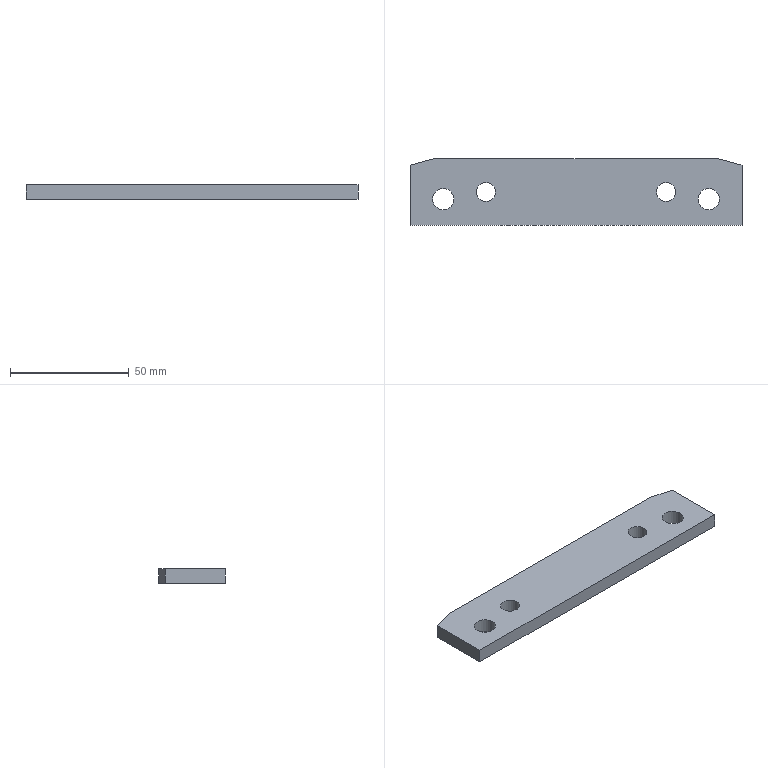Part | STEP file | gslz 2016.10.28-13_id738_x_t | 1 solid | 12 faces | box 140 x 28 x 6 mm | volume 21993 mm3 | plane 8 | cylinder 4 | commonest cylinder face diameters 8 x2 9 x2
STEP:
#1=CARTESIAN_POINT('',(0.,0.,0.));
#2=DIRECTION('',(0.,0.,1.));
#3=DIRECTION('',(1.,0.,0.));
#4=AXIS2_PLACEMENT_3D('',#1,#2,#3);
#5=CARTESIAN_POINT('',(135.484,-281.75,6.));
#6=VERTEX_POINT('',#5);
#7=CARTESIAN_POINT('',(143.484,-281.75,6.));
#8=VERTEX_POINT('',#7);
#9=CARTESIAN_POINT('',(139.484,-281.75,6.));
#10=DIRECTION('',(0.,0.,-1.));
#11=DIRECTION('',(-1.,0.,0.));
#12=AXIS2_PLACEMENT_3D('',#9,#10,#11);
#13=CIRCLE('',#12,4.);
#14=CARTESIAN_POINT('',(139.484,-281.75,-73.));
#15=DIRECTION('',(0.,0.,1.));
#16=DIRECTION('',(1.,0.,0.));
#17=AXIS2_PLACEMENT_3D('',#14,#15,#16);
#18=CYLINDRICAL_SURFACE('',#17,4.);
#19=CARTESIAN_POINT('',(3.142,79.));
#20=DIRECTION('',(-1.,0.));
#21=VECTOR('',#20,1.);
#22=LINE('',#19,#21);
#23=(GEOMETRIC_REPRESENTATION_CONTEXT(2)PARAMETRIC_REPRESENTATION_CONTEXT()REPRESENTATION_CONTEXT('',''));
#24=DEFINITIONAL_REPRESENTATION('',(#22),#23);
#25=PCURVE('',#18,#24);
#26=CARTESIAN_POINT('',(142.484,-265.25,6.));
#27=DIRECTION('',(0.,0.,-1.));
#28=DIRECTION('',(-1.,0.,0.));
#29=AXIS2_PLACEMENT_3D('',#26,#27,#28);
#30=PLANE('',#29);
#31=CARTESIAN_POINT('',(3.,-16.5));
#32=DIRECTION('',(1.,0.));
#33=AXIS2_PLACEMENT_2D('',#31,#32);
#34=CIRCLE('',#33,4.);
#35=(GEOMETRIC_REPRESENTATION_CONTEXT(2)PARAMETRIC_REPRESENTATION_CONTEXT()REPRESENTATION_CONTEXT('',''));
#36=DEFINITIONAL_REPRESENTATION('',(#34),#35);
#37=PCURVE('',#30,#36);
#38=SURFACE_CURVE('',#13,(#25,#37),.PCURVE_S1.);
#39=EDGE_CURVE('',#6,#8,#38,.T.);
#40=ORIENTED_EDGE('',*,*,#39,.T.);
#41=CARTESIAN_POINT('',(143.484,-281.75,0.));
#42=VERTEX_POINT('',#41);
#43=CARTESIAN_POINT('',(143.484,-281.75,0.));
#44=CARTESIAN_POINT('',(143.484,-281.75,6.));
#45=B_SPLINE_CURVE_WITH_KNOTS('',1,(#43,#44),.UNSPECIFIED.,.F.,.F.,(2,2),(73.,79.),.PIECEWISE_BEZIER_KNOTS.);
#46=CARTESIAN_POINT('',(0.,0.));
#47=DIRECTION('',(0.,1.));
#48=VECTOR('',#47,1.);
#49=LINE('',#46,#48);
#50=(GEOMETRIC_REPRESENTATION_CONTEXT(2)PARAMETRIC_REPRESENTATION_CONTEXT()REPRESENTATION_CONTEXT('',''));
#51=DEFINITIONAL_REPRESENTATION('',(#49),#50);
#52=PCURVE('',#18,#51);
#53=CARTESIAN_POINT('',(6.283,0.));
#54=DIRECTION('',(0.,1.));
#55=VECTOR('',#54,1.);
#56=LINE('',#53,#55);
#57=(GEOMETRIC_REPRESENTATION_CONTEXT(2)PARAMETRIC_REPRESENTATION_CONTEXT()REPRESENTATION_CONTEXT('',''));
#58=DEFINITIONAL_REPRESENTATION('',(#56),#57);
#59=PCURVE('',#18,#58);
#60=SEAM_CURVE('',#45,(#52,#59),.PCURVE_S1.);
#61=EDGE_CURVE('',#42,#8,#60,.T.);
#62=ORIENTED_EDGE('',*,*,#61,.F.);
#63=CARTESIAN_POINT('',(139.484,-281.75,0.));
#64=DIRECTION('',(0.,0.,1.));
#65=DIRECTION('',(1.,0.,0.));
#66=AXIS2_PLACEMENT_3D('',#63,#64,#65);
#67=CIRCLE('',#66,4.);
#68=CARTESIAN_POINT('',(0.,73.));
#69=DIRECTION('',(1.,0.));
#70=VECTOR('',#69,1.);
#71=LINE('',#68,#70);
#72=(GEOMETRIC_REPRESENTATION_CONTEXT(2)PARAMETRIC_REPRESENTATION_CONTEXT()REPRESENTATION_CONTEXT('',''));
#73=DEFINITIONAL_REPRESENTATION('',(#71),#72);
#74=PCURVE('',#18,#73);
#75=CARTESIAN_POINT('',(102.484,-295.75,0.));
#76=DIRECTION('',(0.,0.,1.));
#77=DIRECTION('',(1.,0.,0.));
#78=AXIS2_PLACEMENT_3D('',#75,#76,#77);
#79=PLANE('',#78);
#80=CARTESIAN_POINT('',(37.,14.));
#81=DIRECTION('',(1.,0.));
#82=AXIS2_PLACEMENT_2D('',#80,#81);
#83=CIRCLE('',#82,4.);
#84=(GEOMETRIC_REPRESENTATION_CONTEXT(2)PARAMETRIC_REPRESENTATION_CONTEXT()REPRESENTATION_CONTEXT('',''));
#85=DEFINITIONAL_REPRESENTATION('',(#83),#84);
#86=PCURVE('',#79,#85);
#87=SURFACE_CURVE('',#67,(#74,#86),.PCURVE_S1.);
#88=EDGE_CURVE('',#42,#42,#87,.T.);
#89=ORIENTED_EDGE('',*,*,#88,.T.);
#90=ORIENTED_EDGE('',*,*,#61,.T.);
#91=CARTESIAN_POINT('',(139.484,-281.75,6.));
#92=DIRECTION('',(0.,0.,-1.));
#93=DIRECTION('',(-1.,0.,0.));
#94=AXIS2_PLACEMENT_3D('',#91,#92,#93);
#95=CIRCLE('',#94,4.);
#96=CARTESIAN_POINT('',(9.425,79.));
#97=DIRECTION('',(-1.,0.));
#98=VECTOR('',#97,1.);
#99=LINE('',#96,#98);
#100=(GEOMETRIC_REPRESENTATION_CONTEXT(2)PARAMETRIC_REPRESENTATION_CONTEXT()REPRESENTATION_CONTEXT('',''));
#101=DEFINITIONAL_REPRESENTATION('',(#99),#100);
#102=PCURVE('',#18,#101);
#103=CARTESIAN_POINT('',(3.,-16.5));
#104=DIRECTION('',(1.,0.));
#105=AXIS2_PLACEMENT_2D('',#103,#104);
#106=CIRCLE('',#105,4.);
#107=(GEOMETRIC_REPRESENTATION_CONTEXT(2)PARAMETRIC_REPRESENTATION_CONTEXT()REPRESENTATION_CONTEXT('',''));
#108=DEFINITIONAL_REPRESENTATION('',(#106),#107);
#109=PCURVE('',#30,#108);
#110=SURFACE_CURVE('',#95,(#102,#109),.PCURVE_S1.);
#111=EDGE_CURVE('',#8,#6,#110,.T.);
#112=ORIENTED_EDGE('',*,*,#111,.T.);
#113=EDGE_LOOP('',(#40,#62,#89,#90,#112));
#114=FACE_BOUND('',#113,.F.);
#115=ADVANCED_FACE('',(#114),#18,.F.);
#116=CARTESIAN_POINT('',(219.484,-281.75,6.));
#117=VERTEX_POINT('',#116);
#118=CARTESIAN_POINT('',(211.484,-281.75,6.));
#119=VERTEX_POINT('',#118);
#120=CARTESIAN_POINT('',(215.484,-281.75,6.));
#121=DIRECTION('',(0.,0.,1.));
#122=DIRECTION('',(-1.,0.,0.));
#123=AXIS2_PLACEMENT_3D('',#120,#121,#122);
#124=CIRCLE('',#123,4.);
#125=CARTESIAN_POINT('',(215.484,-281.75,-73.));
#126=DIRECTION('',(0.,0.,1.));
#127=DIRECTION('',(1.,0.,0.));
#128=AXIS2_PLACEMENT_3D('',#125,#126,#127);
#129=CYLINDRICAL_SURFACE('',#128,4.);
#130=CARTESIAN_POINT('',(-3.142,79.));
#131=DIRECTION('',(1.,0.));
#132=VECTOR('',#131,1.);
#133=LINE('',#130,#132);
#134=(GEOMETRIC_REPRESENTATION_CONTEXT(2)PARAMETRIC_REPRESENTATION_CONTEXT()REPRESENTATION_CONTEXT('',''));
#135=DEFINITIONAL_REPRESENTATION('',(#133),#134);
#136=PCURVE('',#129,#135);
#137=CARTESIAN_POINT('',(-69.,-16.5));
#138=CARTESIAN_POINT('',(-69.,-23.428));
#139=CARTESIAN_POINT('',(-75.,-19.964));
#140=CARTESIAN_POINT('',(-81.,-16.5));
#141=CARTESIAN_POINT('',(-75.,-13.036));
#142=CARTESIAN_POINT('',(-69.,-9.572));
#143=CARTESIAN_POINT('',(-69.,-16.5));
#144=(BOUNDED_CURVE()B_SPLINE_CURVE(2,(#137,#138,#139,#140,#141,#142,#143),.UNSPECIFIED.,.T.,.F.)B_SPLINE_CURVE_WITH_KNOTS((1,2,2,2,2,1),(-2.094,0.,2.094,4.189,6.283,8.378),.UNSPECIFIED.)CURVE()GEOMETRIC_REPRESENTATION_ITEM()RATIONAL_B_SPLINE_CURVE((1.,0.5,1.,0.5,1.,0.5,1.))REPRESENTATION_ITEM(''));
#145=(GEOMETRIC_REPRESENTATION_CONTEXT(2)PARAMETRIC_REPRESENTATION_CONTEXT()REPRESENTATION_CONTEXT('',''));
#146=DEFINITIONAL_REPRESENTATION('',(#144),#145);
#147=PCURVE('',#30,#146);
#148=SURFACE_CURVE('',#124,(#136,#147),.PCURVE_S1.);
#149=EDGE_CURVE('',#117,#119,#148,.T.);
#150=ORIENTED_EDGE('',*,*,#149,.F.);
#151=CARTESIAN_POINT('',(219.484,-281.75,0.));
#152=VERTEX_POINT('',#151);
#153=CARTESIAN_POINT('',(219.484,-281.75,0.));
#154=CARTESIAN_POINT('',(219.484,-281.75,6.));
#155=B_SPLINE_CURVE_WITH_KNOTS('',1,(#153,#154),.UNSPECIFIED.,.F.,.F.,(2,2),(73.,79.),.PIECEWISE_BEZIER_KNOTS.);
#156=CARTESIAN_POINT('',(0.,0.));
#157=DIRECTION('',(0.,1.));
#158=VECTOR('',#157,1.);
#159=LINE('',#156,#158);
#160=(GEOMETRIC_REPRESENTATION_CONTEXT(2)PARAMETRIC_REPRESENTATION_CONTEXT()REPRESENTATION_CONTEXT('',''));
#161=DEFINITIONAL_REPRESENTATION('',(#159),#160);
#162=PCURVE('',#129,#161);
#163=CARTESIAN_POINT('',(6.283,0.));
#164=DIRECTION('',(0.,1.));
#165=VECTOR('',#164,1.);
#166=LINE('',#163,#165);
#167=(GEOMETRIC_REPRESENTATION_CONTEXT(2)PARAMETRIC_REPRESENTATION_CONTEXT()REPRESENTATION_CONTEXT('',''));
#168=DEFINITIONAL_REPRESENTATION('',(#166),#167);
#169=PCURVE('',#129,#168);
#170=SEAM_CURVE('',#155,(#162,#169),.PCURVE_S1.);
#171=EDGE_CURVE('',#152,#117,#170,.T.);
#172=ORIENTED_EDGE('',*,*,#171,.F.);
#173=CARTESIAN_POINT('',(215.484,-281.75,0.));
#174=DIRECTION('',(0.,0.,-1.));
#175=DIRECTION('',(1.,0.,0.));
#176=AXIS2_PLACEMENT_3D('',#173,#174,#175);
#177=CIRCLE('',#176,4.);
#178=CARTESIAN_POINT('',(6.283,73.));
#179=DIRECTION('',(-1.,0.));
#180=VECTOR('',#179,1.);
#181=LINE('',#178,#180);
#182=(GEOMETRIC_REPRESENTATION_CONTEXT(2)PARAMETRIC_REPRESENTATION_CONTEXT()REPRESENTATION_CONTEXT('',''));
#183=DEFINITIONAL_REPRESENTATION('',(#181),#182);
#184=PCURVE('',#129,#183);
#185=CARTESIAN_POINT('',(117.,14.));
#186=CARTESIAN_POINT('',(117.,7.072));
#187=CARTESIAN_POINT('',(111.,10.536));
#188=CARTESIAN_POINT('',(105.,14.));
#189=CARTESIAN_POINT('',(111.,17.464));
#190=CARTESIAN_POINT('',(117.,20.928));
#191=CARTESIAN_POINT('',(117.,14.));
#192=(BOUNDED_CURVE()B_SPLINE_CURVE(2,(#185,#186,#187,#188,#189,#190,#191),.UNSPECIFIED.,.T.,.F.)B_SPLINE_CURVE_WITH_KNOTS((1,2,2,2,2,1),(-2.094,0.,2.094,4.189,6.283,8.378),.UNSPECIFIED.)CURVE()GEOMETRIC_REPRESENTATION_ITEM()RATIONAL_B_SPLINE_CURVE((1.,0.5,1.,0.5,1.,0.5,1.))REPRESENTATION_ITEM(''));
#193=(GEOMETRIC_REPRESENTATION_CONTEXT(2)PARAMETRIC_REPRESENTATION_CONTEXT()REPRESENTATION_CONTEXT('',''));
#194=DEFINITIONAL_REPRESENTATION('',(#192),#193);
#195=PCURVE('',#79,#194);
#196=SURFACE_CURVE('',#177,(#184,#195),.PCURVE_S1.);
#197=EDGE_CURVE('',#152,#152,#196,.T.);
#198=ORIENTED_EDGE('',*,*,#197,.F.);
#199=ORIENTED_EDGE('',*,*,#171,.T.);
#200=CARTESIAN_POINT('',(215.484,-281.75,6.));
#201=DIRECTION('',(0.,0.,1.));
#202=DIRECTION('',(-1.,0.,0.));
#203=AXIS2_PLACEMENT_3D('',#200,#201,#202);
#204=CIRCLE('',#203,4.);
#205=CARTESIAN_POINT('',(3.142,79.));
#206=DIRECTION('',(1.,0.));
#207=VECTOR('',#206,1.);
#208=LINE('',#205,#207);
#209=(GEOMETRIC_REPRESENTATION_CONTEXT(2)PARAMETRIC_REPRESENTATION_CONTEXT()REPRESENTATION_CONTEXT('',''));
#210=DEFINITIONAL_REPRESENTATION('',(#208),#209);
#211=PCURVE('',#129,#210);
#212=CARTESIAN_POINT('',(-69.,-16.5));
#213=CARTESIAN_POINT('',(-69.,-23.428));
#214=CARTESIAN_POINT('',(-75.,-19.964));
#215=CARTESIAN_POINT('',(-81.,-16.5));
#216=CARTESIAN_POINT('',(-75.,-13.036));
#217=CARTESIAN_POINT('',(-69.,-9.572));
#218=CARTESIAN_POINT('',(-69.,-16.5));
#219=(BOUNDED_CURVE()B_SPLINE_CURVE(2,(#212,#213,#214,#215,#216,#217,#218),.UNSPECIFIED.,.T.,.F.)B_SPLINE_CURVE_WITH_KNOTS((1,2,2,2,2,1),(-2.094,0.,2.094,4.189,6.283,8.378),.UNSPECIFIED.)CURVE()GEOMETRIC_REPRESENTATION_ITEM()RATIONAL_B_SPLINE_CURVE((1.,0.5,1.,0.5,1.,0.5,1.))REPRESENTATION_ITEM(''));
#220=(GEOMETRIC_REPRESENTATION_CONTEXT(2)PARAMETRIC_REPRESENTATION_CONTEXT()REPRESENTATION_CONTEXT('',''));
#221=DEFINITIONAL_REPRESENTATION('',(#219),#220);
#222=PCURVE('',#30,#221);
#223=SURFACE_CURVE('',#204,(#211,#222),.PCURVE_S1.);
#224=EDGE_CURVE('',#119,#117,#223,.T.);
#225=ORIENTED_EDGE('',*,*,#224,.F.);
#226=EDGE_LOOP('',(#150,#172,#198,#199,#225));
#227=FACE_BOUND('',#226,.F.);
#228=ADVANCED_FACE('',(#227),#129,.F.);
#229=CARTESIAN_POINT('',(116.984,-284.75,6.));
#230=VERTEX_POINT('',#229);
#231=CARTESIAN_POINT('',(121.484,-284.75,6.));
#232=DIRECTION('',(0.,0.,1.));
#233=DIRECTION('',(-1.,0.,0.));
#234=AXIS2_PLACEMENT_3D('',#231,#232,#233);
#235=CIRCLE('',#234,4.5);
#236=CARTESIAN_POINT('',(121.484,-284.75,47.));
#237=DIRECTION('',(0.,0.,-1.));
#238=DIRECTION('',(-1.,0.,0.));
#239=AXIS2_PLACEMENT_3D('',#236,#237,#238);
#240=CYLINDRICAL_SURFACE('',#239,4.5);
#241=CARTESIAN_POINT('',(6.283,41.));
#242=DIRECTION('',(-1.,0.));
#243=VECTOR('',#242,1.);
#244=LINE('',#241,#243);
#245=(GEOMETRIC_REPRESENTATION_CONTEXT(2)PARAMETRIC_REPRESENTATION_CONTEXT()REPRESENTATION_CONTEXT('',''));
#246=DEFINITIONAL_REPRESENTATION('',(#244),#245);
#247=PCURVE('',#240,#246);
#248=CARTESIAN_POINT('',(25.5,-19.5));
#249=CARTESIAN_POINT('',(25.5,-27.294));
#250=CARTESIAN_POINT('',(18.75,-23.397));
#251=CARTESIAN_POINT('',(12.,-19.5));
#252=CARTESIAN_POINT('',(18.75,-15.603));
#253=CARTESIAN_POINT('',(25.5,-11.706));
#254=CARTESIAN_POINT('',(25.5,-19.5));
#255=(BOUNDED_CURVE()B_SPLINE_CURVE(2,(#248,#249,#250,#251,#252,#253,#254),.UNSPECIFIED.,.T.,.F.)B_SPLINE_CURVE_WITH_KNOTS((1,2,2,2,2,1),(-2.094,0.,2.094,4.189,6.283,8.378),.UNSPECIFIED.)CURVE()GEOMETRIC_REPRESENTATION_ITEM()RATIONAL_B_SPLINE_CURVE((1.,0.5,1.,0.5,1.,0.5,1.))REPRESENTATION_ITEM(''));
#256=(GEOMETRIC_REPRESENTATION_CONTEXT(2)PARAMETRIC_REPRESENTATION_CONTEXT()REPRESENTATION_CONTEXT('',''));
#257=DEFINITIONAL_REPRESENTATION('',(#255),#256);
#258=PCURVE('',#30,#257);
#259=SURFACE_CURVE('',#235,(#247,#258),.PCURVE_S1.);
#260=EDGE_CURVE('',#230,#230,#259,.T.);
#261=ORIENTED_EDGE('',*,*,#260,.F.);
#262=CARTESIAN_POINT('',(116.984,-284.75,0.));
#263=VERTEX_POINT('',#262);
#264=CARTESIAN_POINT('',(116.984,-284.75,6.));
#265=CARTESIAN_POINT('',(116.984,-284.75,0.));
#266=B_SPLINE_CURVE_WITH_KNOTS('',1,(#264,#265),.UNSPECIFIED.,.F.,.F.,(2,2),(41.,47.),.PIECEWISE_BEZIER_KNOTS.);
#267=CARTESIAN_POINT('',(6.283,0.));
#268=DIRECTION('',(0.,1.));
#269=VECTOR('',#268,1.);
#270=LINE('',#267,#269);
#271=(GEOMETRIC_REPRESENTATION_CONTEXT(2)PARAMETRIC_REPRESENTATION_CONTEXT()REPRESENTATION_CONTEXT('',''));
#272=DEFINITIONAL_REPRESENTATION('',(#270),#271);
#273=PCURVE('',#240,#272);
#274=CARTESIAN_POINT('',(0.,0.));
#275=DIRECTION('',(0.,1.));
#276=VECTOR('',#275,1.);
#277=LINE('',#274,#276);
#278=(GEOMETRIC_REPRESENTATION_CONTEXT(2)PARAMETRIC_REPRESENTATION_CONTEXT()REPRESENTATION_CONTEXT('',''));
#279=DEFINITIONAL_REPRESENTATION('',(#277),#278);
#280=PCURVE('',#240,#279);
#281=SEAM_CURVE('',#266,(#273,#280),.PCURVE_S1.);
#282=EDGE_CURVE('',#230,#263,#281,.T.);
#283=ORIENTED_EDGE('',*,*,#282,.T.);
#284=CARTESIAN_POINT('',(125.984,-284.75,0.));
#285=VERTEX_POINT('',#284);
#286=CARTESIAN_POINT('',(121.484,-284.75,0.));
#287=DIRECTION('',(0.,0.,-1.));
#288=DIRECTION('',(1.,0.,0.));
#289=AXIS2_PLACEMENT_3D('',#286,#287,#288);
#290=CIRCLE('',#289,4.5);
#291=CARTESIAN_POINT('',(3.142,47.));
#292=DIRECTION('',(1.,0.));
#293=VECTOR('',#292,1.);
#294=LINE('',#291,#293);
#295=(GEOMETRIC_REPRESENTATION_CONTEXT(2)PARAMETRIC_REPRESENTATION_CONTEXT()REPRESENTATION_CONTEXT('',''));
#296=DEFINITIONAL_REPRESENTATION('',(#294),#295);
#297=PCURVE('',#240,#296);
#298=CARTESIAN_POINT('',(23.5,11.));
#299=CARTESIAN_POINT('',(23.5,3.206));
#300=CARTESIAN_POINT('',(16.75,7.103));
#301=CARTESIAN_POINT('',(10.,11.));
#302=CARTESIAN_POINT('',(16.75,14.897));
#303=CARTESIAN_POINT('',(23.5,18.794));
#304=CARTESIAN_POINT('',(23.5,11.));
#305=(BOUNDED_CURVE()B_SPLINE_CURVE(2,(#298,#299,#300,#301,#302,#303,#304),.UNSPECIFIED.,.T.,.F.)B_SPLINE_CURVE_WITH_KNOTS((1,2,2,2,2,1),(-2.094,0.,2.094,4.189,6.283,8.378),.UNSPECIFIED.)CURVE()GEOMETRIC_REPRESENTATION_ITEM()RATIONAL_B_SPLINE_CURVE((1.,0.5,1.,0.5,1.,0.5,1.))REPRESENTATION_ITEM(''));
#306=(GEOMETRIC_REPRESENTATION_CONTEXT(2)PARAMETRIC_REPRESENTATION_CONTEXT()REPRESENTATION_CONTEXT('',''));
#307=DEFINITIONAL_REPRESENTATION('',(#305),#306);
#308=PCURVE('',#79,#307);
#309=SURFACE_CURVE('',#290,(#297,#308),.PCURVE_S1.);
#310=EDGE_CURVE('',#285,#263,#309,.T.);
#311=ORIENTED_EDGE('',*,*,#310,.F.);
#312=CARTESIAN_POINT('',(121.484,-284.75,0.));
#313=DIRECTION('',(0.,0.,-1.));
#314=DIRECTION('',(1.,0.,0.));
#315=AXIS2_PLACEMENT_3D('',#312,#313,#314);
#316=CIRCLE('',#315,4.5);
#317=CARTESIAN_POINT('',(-3.142,47.));
#318=DIRECTION('',(1.,0.));
#319=VECTOR('',#318,1.);
#320=LINE('',#317,#319);
#321=(GEOMETRIC_REPRESENTATION_CONTEXT(2)PARAMETRIC_REPRESENTATION_CONTEXT()REPRESENTATION_CONTEXT('',''));
#322=DEFINITIONAL_REPRESENTATION('',(#320),#321);
#323=PCURVE('',#240,#322);
#324=CARTESIAN_POINT('',(23.5,11.));
#325=CARTESIAN_POINT('',(23.5,3.206));
#326=CARTESIAN_POINT('',(16.75,7.103));
#327=CARTESIAN_POINT('',(10.,11.));
#328=CARTESIAN_POINT('',(16.75,14.897));
#329=CARTESIAN_POINT('',(23.5,18.794));
#330=CARTESIAN_POINT('',(23.5,11.));
#331=(BOUNDED_CURVE()B_SPLINE_CURVE(2,(#324,#325,#326,#327,#328,#329,#330),.UNSPECIFIED.,.T.,.F.)B_SPLINE_CURVE_WITH_KNOTS((1,2,2,2,2,1),(-2.094,0.,2.094,4.189,6.283,8.378),.UNSPECIFIED.)CURVE()GEOMETRIC_REPRESENTATION_ITEM()RATIONAL_B_SPLINE_CURVE((1.,0.5,1.,0.5,1.,0.5,1.))REPRESENTATION_ITEM(''));
#332=(GEOMETRIC_REPRESENTATION_CONTEXT(2)PARAMETRIC_REPRESENTATION_CONTEXT()REPRESENTATION_CONTEXT('',''));
#333=DEFINITIONAL_REPRESENTATION('',(#331),#332);
#334=PCURVE('',#79,#333);
#335=SURFACE_CURVE('',#316,(#323,#334),.PCURVE_S1.);
#336=EDGE_CURVE('',#263,#285,#335,.T.);
#337=ORIENTED_EDGE('',*,*,#336,.F.);
#338=ORIENTED_EDGE('',*,*,#282,.F.);
#339=EDGE_LOOP('',(#261,#283,#311,#337,#338));
#340=FACE_BOUND('',#339,.F.);
#341=ADVANCED_FACE('',(#340),#240,.F.);
#342=CARTESIAN_POINT('',(237.485,-267.75,0.));
#343=VERTEX_POINT('',#342);
#344=CARTESIAN_POINT('',(237.485,-267.75,6.));
#345=VERTEX_POINT('',#344);
#346=CARTESIAN_POINT('',(237.485,-267.75,8.));
#347=DIRECTION('',(0.,0.,1.));
#348=VECTOR('',#347,1.);
#349=LINE('',#346,#348);
#350=CARTESIAN_POINT('',(112.486,-267.75,8.));
#351=DIRECTION('',(0.,-1.,0.));
#352=DIRECTION('',(0.,0.,1.));
#353=AXIS2_PLACEMENT_3D('',#350,#351,#352);
#354=PLANE('',#353);
#355=CARTESIAN_POINT('',(0.,-124.999));
#356=DIRECTION('',(1.,0.));
#357=VECTOR('',#356,1.);
#358=LINE('',#355,#357);
#359=(GEOMETRIC_REPRESENTATION_CONTEXT(2)PARAMETRIC_REPRESENTATION_CONTEXT()REPRESENTATION_CONTEXT('',''));
#360=DEFINITIONAL_REPRESENTATION('',(#358),#359);
#361=PCURVE('',#354,#360);
#362=CARTESIAN_POINT('',(237.485,-267.75,8.));
#363=DIRECTION('',(-0.2588,-0.9659,0.));
#364=DIRECTION('',(-0.9659,0.2588,0.));
#365=AXIS2_PLACEMENT_3D('',#362,#363,#364);
#366=PLANE('',#365);
#367=CARTESIAN_POINT('',(0.,0.));
#368=DIRECTION('',(0.,-1.));
#369=VECTOR('',#368,1.);
#370=LINE('',#367,#369);
#371=(GEOMETRIC_REPRESENTATION_CONTEXT(2)PARAMETRIC_REPRESENTATION_CONTEXT()REPRESENTATION_CONTEXT('',''));
#372=DEFINITIONAL_REPRESENTATION('',(#370),#371);
#373=PCURVE('',#366,#372);
#374=SURFACE_CURVE('',#349,(#361,#373),.PCURVE_S1.);
#375=EDGE_CURVE('',#343,#345,#374,.T.);
#376=ORIENTED_EDGE('',*,*,#375,.F.);
#377=CARTESIAN_POINT('',(117.486,-267.75,0.));
#378=VERTEX_POINT('',#377);
#379=CARTESIAN_POINT('',(112.486,-267.75,0.));
#380=DIRECTION('',(1.,0.,0.));
#381=VECTOR('',#380,1.);
#382=LINE('',#379,#381);
#383=CARTESIAN_POINT('',(-8.,0.));
#384=DIRECTION('',(0.,-1.));
#385=VECTOR('',#384,1.);
#386=LINE('',#383,#385);
#387=(GEOMETRIC_REPRESENTATION_CONTEXT(2)PARAMETRIC_REPRESENTATION_CONTEXT()REPRESENTATION_CONTEXT('',''));
#388=DEFINITIONAL_REPRESENTATION('',(#386),#387);
#389=PCURVE('',#354,#388);
#390=CARTESIAN_POINT('',(10.002,28.));
#391=DIRECTION('',(1.,0.));
#392=VECTOR('',#391,1.);
#393=LINE('',#390,#392);
#394=(GEOMETRIC_REPRESENTATION_CONTEXT(2)PARAMETRIC_REPRESENTATION_CONTEXT()REPRESENTATION_CONTEXT('',''));
#395=DEFINITIONAL_REPRESENTATION('',(#393),#394);
#396=PCURVE('',#79,#395);
#397=SURFACE_CURVE('',#382,(#389,#396),.PCURVE_S1.);
#398=EDGE_CURVE('',#378,#343,#397,.T.);
#399=ORIENTED_EDGE('',*,*,#398,.F.);
#400=CARTESIAN_POINT('',(117.486,-267.75,6.));
#401=VERTEX_POINT('',#400);
#402=CARTESIAN_POINT('',(117.486,-267.75,8.));
#403=DIRECTION('',(0.,0.,1.));
#404=VECTOR('',#403,1.);
#405=LINE('',#402,#404);
#406=CARTESIAN_POINT('',(0.,-5.));
#407=DIRECTION('',(1.,0.));
#408=VECTOR('',#407,1.);
#409=LINE('',#406,#408);
#410=(GEOMETRIC_REPRESENTATION_CONTEXT(2)PARAMETRIC_REPRESENTATION_CONTEXT()REPRESENTATION_CONTEXT('',''));
#411=DEFINITIONAL_REPRESENTATION('',(#409),#410);
#412=PCURVE('',#354,#411);
#413=CARTESIAN_POINT('',(107.484,-270.43,8.));
#414=DIRECTION('',(0.2588,-0.9659,0.));
#415=DIRECTION('',(-0.9659,-0.2588,0.));
#416=AXIS2_PLACEMENT_3D('',#413,#414,#415);
#417=PLANE('',#416);
#418=CARTESIAN_POINT('',(-10.355,0.));
#419=DIRECTION('',(0.,-1.));
#420=VECTOR('',#419,1.);
#421=LINE('',#418,#420);
#422=(GEOMETRIC_REPRESENTATION_CONTEXT(2)PARAMETRIC_REPRESENTATION_CONTEXT()REPRESENTATION_CONTEXT('',''));
#423=DEFINITIONAL_REPRESENTATION('',(#421),#422);
#424=PCURVE('',#417,#423);
#425=SURFACE_CURVE('',#405,(#412,#424),.PCURVE_S1.);
#426=EDGE_CURVE('',#378,#401,#425,.T.);
#427=ORIENTED_EDGE('',*,*,#426,.T.);
#428=CARTESIAN_POINT('',(112.486,-267.75,6.));
#429=DIRECTION('',(-1.,0.,0.));
#430=VECTOR('',#429,1.);
#431=LINE('',#428,#430);
#432=CARTESIAN_POINT('',(-2.,0.));
#433=DIRECTION('',(0.,1.));
#434=VECTOR('',#433,1.);
#435=LINE('',#432,#434);
#436=(GEOMETRIC_REPRESENTATION_CONTEXT(2)PARAMETRIC_REPRESENTATION_CONTEXT()REPRESENTATION_CONTEXT('',''));
#437=DEFINITIONAL_REPRESENTATION('',(#435),#436);
#438=PCURVE('',#354,#437);
#439=CARTESIAN_POINT('',(29.998,-2.5));
#440=DIRECTION('',(1.,0.));
#441=VECTOR('',#440,1.);
#442=LINE('',#439,#441);
#443=(GEOMETRIC_REPRESENTATION_CONTEXT(2)PARAMETRIC_REPRESENTATION_CONTEXT()REPRESENTATION_CONTEXT('',''));
#444=DEFINITIONAL_REPRESENTATION('',(#442),#443);
#445=PCURVE('',#30,#444);
#446=SURFACE_CURVE('',#431,(#438,#445),.PCURVE_S1.);
#447=EDGE_CURVE('',#345,#401,#446,.T.);
#448=ORIENTED_EDGE('',*,*,#447,.F.);
#449=EDGE_LOOP('',(#376,#399,#427,#448));
#450=FACE_BOUND('',#449,.T.);
#451=ADVANCED_FACE('',(#450),#354,.F.);
#452=CARTESIAN_POINT('',(247.484,-270.429,6.));
#453=VERTEX_POINT('',#452);
#454=CARTESIAN_POINT('',(247.484,-270.429,0.));
#455=VERTEX_POINT('',#454);
#456=CARTESIAN_POINT('',(247.484,-270.429,8.));
#457=DIRECTION('',(0.,0.,-1.));
#458=VECTOR('',#457,1.);
#459=LINE('',#456,#458);
#460=CARTESIAN_POINT('',(-10.352,0.));
#461=DIRECTION('',(0.,1.));
#462=VECTOR('',#461,1.);
#463=LINE('',#460,#462);
#464=(GEOMETRIC_REPRESENTATION_CONTEXT(2)PARAMETRIC_REPRESENTATION_CONTEXT()REPRESENTATION_CONTEXT('',''));
#465=DEFINITIONAL_REPRESENTATION('',(#463),#464);
#466=PCURVE('',#366,#465);
#467=CARTESIAN_POINT('',(247.484,-262.75,16.));
#468=DIRECTION('',(-1.,0.,0.));
#469=DIRECTION('',(0.,0.,1.));
#470=AXIS2_PLACEMENT_3D('',#467,#468,#469);
#471=PLANE('',#470);
#472=CARTESIAN_POINT('',(-8.,-7.679));
#473=DIRECTION('',(-1.,0.));
#474=VECTOR('',#473,1.);
#475=LINE('',#472,#474);
#476=(GEOMETRIC_REPRESENTATION_CONTEXT(2)PARAMETRIC_REPRESENTATION_CONTEXT()REPRESENTATION_CONTEXT('',''));
#477=DEFINITIONAL_REPRESENTATION('',(#475),#476);
#478=PCURVE('',#471,#477);
#479=SURFACE_CURVE('',#459,(#466,#478),.PCURVE_S1.);
#480=EDGE_CURVE('',#453,#455,#479,.T.);
#481=ORIENTED_EDGE('',*,*,#480,.T.);
#482=CARTESIAN_POINT('',(237.485,-267.75,0.));
#483=DIRECTION('',(0.9659,-0.2588,0.));
#484=VECTOR('',#483,1.);
#485=LINE('',#482,#484);
#486=CARTESIAN_POINT('',(0.,8.));
#487=DIRECTION('',(-1.,0.));
#488=VECTOR('',#487,1.);
#489=LINE('',#486,#488);
#490=(GEOMETRIC_REPRESENTATION_CONTEXT(2)PARAMETRIC_REPRESENTATION_CONTEXT()REPRESENTATION_CONTEXT('',''));
#491=DEFINITIONAL_REPRESENTATION('',(#489),#490);
#492=PCURVE('',#366,#491);
#493=CARTESIAN_POINT('',(135.001,28.));
#494=DIRECTION('',(0.9659,-0.2588));
#495=VECTOR('',#494,1.);
#496=LINE('',#493,#495);
#497=(GEOMETRIC_REPRESENTATION_CONTEXT(2)PARAMETRIC_REPRESENTATION_CONTEXT()REPRESENTATION_CONTEXT('',''));
#498=DEFINITIONAL_REPRESENTATION('',(#496),#497);
#499=PCURVE('',#79,#498);
#500=SURFACE_CURVE('',#485,(#492,#499),.PCURVE_S1.);
#501=EDGE_CURVE('',#343,#455,#500,.T.);
#502=ORIENTED_EDGE('',*,*,#501,.F.);
#503=ORIENTED_EDGE('',*,*,#375,.T.);
#504=CARTESIAN_POINT('',(237.485,-267.75,6.));
#505=DIRECTION('',(-0.9659,0.2588,0.));
#506=VECTOR('',#505,1.);
#507=LINE('',#504,#506);
#508=CARTESIAN_POINT('',(0.,2.));
#509=DIRECTION('',(1.,0.));
#510=VECTOR('',#509,1.);
#511=LINE('',#508,#510);
#512=(GEOMETRIC_REPRESENTATION_CONTEXT(2)PARAMETRIC_REPRESENTATION_CONTEXT()REPRESENTATION_CONTEXT('',''));
#513=DEFINITIONAL_REPRESENTATION('',(#511),#512);
#514=PCURVE('',#366,#513);
#515=CARTESIAN_POINT('',(-95.001,-2.5));
#516=DIRECTION('',(0.9659,0.2588));
#517=VECTOR('',#516,1.);
#518=LINE('',#515,#517);
#519=(GEOMETRIC_REPRESENTATION_CONTEXT(2)PARAMETRIC_REPRESENTATION_CONTEXT()REPRESENTATION_CONTEXT('',''));
#520=DEFINITIONAL_REPRESENTATION('',(#518),#519);
#521=PCURVE('',#30,#520);
#522=SURFACE_CURVE('',#507,(#514,#521),.PCURVE_S1.);
#523=EDGE_CURVE('',#453,#345,#522,.T.);
#524=ORIENTED_EDGE('',*,*,#523,.F.);
#525=EDGE_LOOP('',(#481,#502,#503,#524));
#526=FACE_BOUND('',#525,.T.);
#527=ADVANCED_FACE('',(#526),#366,.F.);
#528=CARTESIAN_POINT('',(247.484,-295.75,6.));
#529=VERTEX_POINT('',#528);
#530=CARTESIAN_POINT('',(247.484,-295.75,0.));
#531=VERTEX_POINT('',#530);
#532=CARTESIAN_POINT('',(247.484,-295.75,16.));
#533=DIRECTION('',(0.,0.,-1.));
#534=VECTOR('',#533,1.);
#535=LINE('',#532,#534);
#536=CARTESIAN_POINT('',(0.,-33.));
#537=DIRECTION('',(-1.,0.));
#538=VECTOR('',#537,1.);
#539=LINE('',#536,#538);
#540=(GEOMETRIC_REPRESENTATION_CONTEXT(2)PARAMETRIC_REPRESENTATION_CONTEXT()REPRESENTATION_CONTEXT('',''));
#541=DEFINITIONAL_REPRESENTATION('',(#539),#540);
#542=PCURVE('',#471,#541);
#543=CARTESIAN_POINT('',(182.484,-295.75,16.));
#544=DIRECTION('',(0.,1.,0.));
#545=DIRECTION('',(0.,0.,-1.));
#546=AXIS2_PLACEMENT_3D('',#543,#544,#545);
#547=PLANE('',#546);
#548=CARTESIAN_POINT('',(0.,-65.));
#549=DIRECTION('',(1.,0.));
#550=VECTOR('',#549,1.);
#551=LINE('',#548,#550);
#552=(GEOMETRIC_REPRESENTATION_CONTEXT(2)PARAMETRIC_REPRESENTATION_CONTEXT()REPRESENTATION_CONTEXT('',''));
#553=DEFINITIONAL_REPRESENTATION('',(#551),#552);
#554=PCURVE('',#547,#553);
#555=SURFACE_CURVE('',#535,(#542,#554),.PCURVE_S1.);
#556=EDGE_CURVE('',#529,#531,#555,.T.);
#557=ORIENTED_EDGE('',*,*,#556,.T.);
#558=CARTESIAN_POINT('',(247.484,-262.75,0.));
#559=DIRECTION('',(0.,-1.,0.));
#560=VECTOR('',#559,1.);
#561=LINE('',#558,#560);
#562=CARTESIAN_POINT('',(-16.,0.));
#563=DIRECTION('',(0.,-1.));
#564=VECTOR('',#563,1.);
#565=LINE('',#562,#564);
#566=(GEOMETRIC_REPRESENTATION_CONTEXT(2)PARAMETRIC_REPRESENTATION_CONTEXT()REPRESENTATION_CONTEXT('',''));
#567=DEFINITIONAL_REPRESENTATION('',(#565),#566);
#568=PCURVE('',#471,#567);
#569=CARTESIAN_POINT('',(145.,33.));
#570=DIRECTION('',(0.,-1.));
#571=VECTOR('',#570,1.);
#572=LINE('',#569,#571);
#573=(GEOMETRIC_REPRESENTATION_CONTEXT(2)PARAMETRIC_REPRESENTATION_CONTEXT()REPRESENTATION_CONTEXT('',''));
#574=DEFINITIONAL_REPRESENTATION('',(#572),#573);
#575=PCURVE('',#79,#574);
#576=SURFACE_CURVE('',#561,(#568,#575),.PCURVE_S1.);
#577=EDGE_CURVE('',#455,#531,#576,.T.);
#578=ORIENTED_EDGE('',*,*,#577,.F.);
#579=ORIENTED_EDGE('',*,*,#480,.F.);
#580=CARTESIAN_POINT('',(247.484,-262.75,6.));
#581=DIRECTION('',(0.,1.,0.));
#582=VECTOR('',#581,1.);
#583=LINE('',#580,#582);
#584=CARTESIAN_POINT('',(-10.,0.));
#585=DIRECTION('',(0.,1.));
#586=VECTOR('',#585,1.);
#587=LINE('',#584,#586);
#588=(GEOMETRIC_REPRESENTATION_CONTEXT(2)PARAMETRIC_REPRESENTATION_CONTEXT()REPRESENTATION_CONTEXT('',''));
#589=DEFINITIONAL_REPRESENTATION('',(#587),#588);
#590=PCURVE('',#471,#589);
#591=CARTESIAN_POINT('',(-105.,2.5));
#592=DIRECTION('',(0.,1.));
#593=VECTOR('',#592,1.);
#594=LINE('',#591,#593);
#595=(GEOMETRIC_REPRESENTATION_CONTEXT(2)PARAMETRIC_REPRESENTATION_CONTEXT()REPRESENTATION_CONTEXT('',''));
#596=DEFINITIONAL_REPRESENTATION('',(#594),#595);
#597=PCURVE('',#30,#596);
#598=SURFACE_CURVE('',#583,(#590,#597),.PCURVE_S1.);
#599=EDGE_CURVE('',#529,#453,#598,.T.);
#600=ORIENTED_EDGE('',*,*,#599,.F.);
#601=EDGE_LOOP('',(#557,#578,#579,#600));
#602=FACE_BOUND('',#601,.T.);
#603=ADVANCED_FACE('',(#602),#471,.F.);
#604=CARTESIAN_POINT('',(107.484,-295.75,6.));
#605=VERTEX_POINT('',#604);
#606=CARTESIAN_POINT('',(107.484,-295.75,0.));
#607=VERTEX_POINT('',#606);
#608=CARTESIAN_POINT('',(107.484,-295.75,16.));
#609=DIRECTION('',(0.,0.,-1.));
#610=VECTOR('',#609,1.);
#611=LINE('',#608,#610);
#612=CARTESIAN_POINT('',(0.,75.));
#613=DIRECTION('',(1.,0.));
#614=VECTOR('',#613,1.);
#615=LINE('',#612,#614);
#616=(GEOMETRIC_REPRESENTATION_CONTEXT(2)PARAMETRIC_REPRESENTATION_CONTEXT()REPRESENTATION_CONTEXT('',''));
#617=DEFINITIONAL_REPRESENTATION('',(#615),#616);
#618=PCURVE('',#547,#617);
#619=CARTESIAN_POINT('',(107.484,-295.75,16.));
#620=DIRECTION('',(1.,0.,0.));
#621=DIRECTION('',(0.,0.,-1.));
#622=AXIS2_PLACEMENT_3D('',#619,#620,#621);
#623=PLANE('',#622);
#624=CARTESIAN_POINT('',(0.,0.));
#625=DIRECTION('',(1.,0.));
#626=VECTOR('',#625,1.);
#627=LINE('',#624,#626);
#628=(GEOMETRIC_REPRESENTATION_CONTEXT(2)PARAMETRIC_REPRESENTATION_CONTEXT()REPRESENTATION_CONTEXT('',''));
#629=DEFINITIONAL_REPRESENTATION('',(#627),#628);
#630=PCURVE('',#623,#629);
#631=SURFACE_CURVE('',#611,(#618,#630),.PCURVE_S1.);
#632=EDGE_CURVE('',#605,#607,#631,.T.);
#633=ORIENTED_EDGE('',*,*,#632,.T.);
#634=CARTESIAN_POINT('',(182.484,-295.75,0.));
#635=DIRECTION('',(-1.,0.,0.));
#636=VECTOR('',#635,1.);
#637=LINE('',#634,#636);
#638=CARTESIAN_POINT('',(16.,0.));
#639=DIRECTION('',(0.,1.));
#640=VECTOR('',#639,1.);
#641=LINE('',#638,#640);
#642=(GEOMETRIC_REPRESENTATION_CONTEXT(2)PARAMETRIC_REPRESENTATION_CONTEXT()REPRESENTATION_CONTEXT('',''));
#643=DEFINITIONAL_REPRESENTATION('',(#641),#642);
#644=PCURVE('',#547,#643);
#645=CARTESIAN_POINT('',(80.,0.));
#646=DIRECTION('',(-1.,0.));
#647=VECTOR('',#646,1.);
#648=LINE('',#645,#647);
#649=(GEOMETRIC_REPRESENTATION_CONTEXT(2)PARAMETRIC_REPRESENTATION_CONTEXT()REPRESENTATION_CONTEXT('',''));
#650=DEFINITIONAL_REPRESENTATION('',(#648),#649);
#651=PCURVE('',#79,#650);
#652=SURFACE_CURVE('',#637,(#644,#651),.PCURVE_S1.);
#653=EDGE_CURVE('',#531,#607,#652,.T.);
#654=ORIENTED_EDGE('',*,*,#653,.F.);
#655=ORIENTED_EDGE('',*,*,#556,.F.);
#656=CARTESIAN_POINT('',(182.484,-295.75,6.));
#657=DIRECTION('',(1.,0.,0.));
#658=VECTOR('',#657,1.);
#659=LINE('',#656,#658);
#660=CARTESIAN_POINT('',(10.,0.));
#661=DIRECTION('',(0.,-1.));
#662=VECTOR('',#661,1.);
#663=LINE('',#660,#662);
#664=(GEOMETRIC_REPRESENTATION_CONTEXT(2)PARAMETRIC_REPRESENTATION_CONTEXT()REPRESENTATION_CONTEXT('',''));
#665=DEFINITIONAL_REPRESENTATION('',(#663),#664);
#666=PCURVE('',#547,#665);
#667=CARTESIAN_POINT('',(-40.,-30.5));
#668=DIRECTION('',(-1.,0.));
#669=VECTOR('',#668,1.);
#670=LINE('',#667,#669);
#671=(GEOMETRIC_REPRESENTATION_CONTEXT(2)PARAMETRIC_REPRESENTATION_CONTEXT()REPRESENTATION_CONTEXT('',''));
#672=DEFINITIONAL_REPRESENTATION('',(#670),#671);
#673=PCURVE('',#30,#672);
#674=SURFACE_CURVE('',#659,(#666,#673),.PCURVE_S1.);
#675=EDGE_CURVE('',#605,#529,#674,.T.);
#676=ORIENTED_EDGE('',*,*,#675,.F.);
#677=EDGE_LOOP('',(#633,#654,#655,#676));
#678=FACE_BOUND('',#677,.T.);
#679=ADVANCED_FACE('',(#678),#547,.F.);
#680=CARTESIAN_POINT('',(107.484,-270.43,6.));
#681=VERTEX_POINT('',#680);
#682=CARTESIAN_POINT('',(107.484,-270.43,0.));
#683=VERTEX_POINT('',#682);
#684=CARTESIAN_POINT('',(107.484,-270.43,8.));
#685=DIRECTION('',(0.,0.,-1.));
#686=VECTOR('',#685,1.);
#687=LINE('',#684,#686);
#688=CARTESIAN_POINT('',(8.,25.32));
#689=DIRECTION('',(1.,0.));
#690=VECTOR('',#689,1.);
#691=LINE('',#688,#690);
#692=(GEOMETRIC_REPRESENTATION_CONTEXT(2)PARAMETRIC_REPRESENTATION_CONTEXT()REPRESENTATION_CONTEXT('',''));
#693=DEFINITIONAL_REPRESENTATION('',(#691),#692);
#694=PCURVE('',#623,#693);
#695=CARTESIAN_POINT('',(0.,0.));
#696=DIRECTION('',(0.,1.));
#697=VECTOR('',#696,1.);
#698=LINE('',#695,#697);
#699=(GEOMETRIC_REPRESENTATION_CONTEXT(2)PARAMETRIC_REPRESENTATION_CONTEXT()REPRESENTATION_CONTEXT('',''));
#700=DEFINITIONAL_REPRESENTATION('',(#698),#699);
#701=PCURVE('',#417,#700);
#702=SURFACE_CURVE('',#687,(#694,#701),.PCURVE_S1.);
#703=EDGE_CURVE('',#681,#683,#702,.T.);
#704=ORIENTED_EDGE('',*,*,#703,.T.);
#705=CARTESIAN_POINT('',(107.484,-295.75,0.));
#706=DIRECTION('',(0.,1.,0.));
#707=VECTOR('',#706,1.);
#708=LINE('',#705,#707);
#709=CARTESIAN_POINT('',(16.,0.));
#710=DIRECTION('',(0.,1.));
#711=VECTOR('',#710,1.);
#712=LINE('',#709,#711);
#713=(GEOMETRIC_REPRESENTATION_CONTEXT(2)PARAMETRIC_REPRESENTATION_CONTEXT()REPRESENTATION_CONTEXT('',''));
#714=DEFINITIONAL_REPRESENTATION('',(#712),#713);
#715=PCURVE('',#623,#714);
#716=CARTESIAN_POINT('',(5.,0.));
#717=DIRECTION('',(0.,1.));
#718=VECTOR('',#717,1.);
#719=LINE('',#716,#718);
#720=(GEOMETRIC_REPRESENTATION_CONTEXT(2)PARAMETRIC_REPRESENTATION_CONTEXT()REPRESENTATION_CONTEXT('',''));
#721=DEFINITIONAL_REPRESENTATION('',(#719),#720);
#722=PCURVE('',#79,#721);
#723=SURFACE_CURVE('',#708,(#715,#722),.PCURVE_S1.);
#724=EDGE_CURVE('',#607,#683,#723,.T.);
#725=ORIENTED_EDGE('',*,*,#724,.F.);
#726=ORIENTED_EDGE('',*,*,#632,.F.);
#727=CARTESIAN_POINT('',(107.484,-295.75,6.));
#728=DIRECTION('',(0.,-1.,0.));
#729=VECTOR('',#728,1.);
#730=LINE('',#727,#729);
#731=CARTESIAN_POINT('',(10.,0.));
#732=DIRECTION('',(0.,-1.));
#733=VECTOR('',#732,1.);
#734=LINE('',#731,#733);
#735=(GEOMETRIC_REPRESENTATION_CONTEXT(2)PARAMETRIC_REPRESENTATION_CONTEXT()REPRESENTATION_CONTEXT('',''));
#736=DEFINITIONAL_REPRESENTATION('',(#734),#735);
#737=PCURVE('',#623,#736);
#738=CARTESIAN_POINT('',(35.,-30.5));
#739=DIRECTION('',(0.,-1.));
#740=VECTOR('',#739,1.);
#741=LINE('',#738,#740);
#742=(GEOMETRIC_REPRESENTATION_CONTEXT(2)PARAMETRIC_REPRESENTATION_CONTEXT()REPRESENTATION_CONTEXT('',''));
#743=DEFINITIONAL_REPRESENTATION('',(#741),#742);
#744=PCURVE('',#30,#743);
#745=SURFACE_CURVE('',#730,(#737,#744),.PCURVE_S1.);
#746=EDGE_CURVE('',#681,#605,#745,.T.);
#747=ORIENTED_EDGE('',*,*,#746,.F.);
#748=EDGE_LOOP('',(#704,#725,#726,#747));
#749=FACE_BOUND('',#748,.T.);
#750=ADVANCED_FACE('',(#749),#623,.F.);
#751=ORIENTED_EDGE('',*,*,#426,.F.);
#752=CARTESIAN_POINT('',(107.484,-270.43,0.));
#753=DIRECTION('',(0.9659,0.2588,0.));
#754=VECTOR('',#753,1.);
#755=LINE('',#752,#754);
#756=CARTESIAN_POINT('',(0.,8.));
#757=DIRECTION('',(-1.,0.));
#758=VECTOR('',#757,1.);
#759=LINE('',#756,#758);
#760=(GEOMETRIC_REPRESENTATION_CONTEXT(2)PARAMETRIC_REPRESENTATION_CONTEXT()REPRESENTATION_CONTEXT('',''));
#761=DEFINITIONAL_REPRESENTATION('',(#759),#760);
#762=PCURVE('',#417,#761);
#763=CARTESIAN_POINT('',(5.,25.32));
#764=DIRECTION('',(0.9659,0.2588));
#765=VECTOR('',#764,1.);
#766=LINE('',#763,#765);
#767=(GEOMETRIC_REPRESENTATION_CONTEXT(2)PARAMETRIC_REPRESENTATION_CONTEXT()REPRESENTATION_CONTEXT('',''));
#768=DEFINITIONAL_REPRESENTATION('',(#766),#767);
#769=PCURVE('',#79,#768);
#770=SURFACE_CURVE('',#755,(#762,#769),.PCURVE_S1.);
#771=EDGE_CURVE('',#683,#378,#770,.T.);
#772=ORIENTED_EDGE('',*,*,#771,.F.);
#773=ORIENTED_EDGE('',*,*,#703,.F.);
#774=CARTESIAN_POINT('',(107.484,-270.43,6.));
#775=DIRECTION('',(-0.9659,-0.2588,0.));
#776=VECTOR('',#775,1.);
#777=LINE('',#774,#776);
#778=CARTESIAN_POINT('',(0.,2.));
#779=DIRECTION('',(1.,0.));
#780=VECTOR('',#779,1.);
#781=LINE('',#778,#780);
#782=(GEOMETRIC_REPRESENTATION_CONTEXT(2)PARAMETRIC_REPRESENTATION_CONTEXT()REPRESENTATION_CONTEXT('',''));
#783=DEFINITIONAL_REPRESENTATION('',(#781),#782);
#784=PCURVE('',#417,#783);
#785=CARTESIAN_POINT('',(35.,-5.18));
#786=DIRECTION('',(0.9659,-0.2588));
#787=VECTOR('',#786,1.);
#788=LINE('',#785,#787);
#789=(GEOMETRIC_REPRESENTATION_CONTEXT(2)PARAMETRIC_REPRESENTATION_CONTEXT()REPRESENTATION_CONTEXT('',''));
#790=DEFINITIONAL_REPRESENTATION('',(#788),#789);
#791=PCURVE('',#30,#790);
#792=SURFACE_CURVE('',#777,(#784,#791),.PCURVE_S1.);
#793=EDGE_CURVE('',#401,#681,#792,.T.);
#794=ORIENTED_EDGE('',*,*,#793,.F.);
#795=EDGE_LOOP('',(#751,#772,#773,#794));
#796=FACE_BOUND('',#795,.T.);
#797=ADVANCED_FACE('',(#796),#417,.F.);
#798=ORIENTED_EDGE('',*,*,#771,.T.);
#799=ORIENTED_EDGE('',*,*,#398,.T.);
#800=ORIENTED_EDGE('',*,*,#501,.T.);
#801=ORIENTED_EDGE('',*,*,#577,.T.);
#802=ORIENTED_EDGE('',*,*,#653,.T.);
#803=ORIENTED_EDGE('',*,*,#724,.T.);
#804=EDGE_LOOP('',(#798,#799,#800,#801,#802,#803));
#805=FACE_BOUND('',#804,.T.);
#806=ORIENTED_EDGE('',*,*,#310,.F.);
#807=ORIENTED_EDGE('',*,*,#336,.F.);
#808=EDGE_LOOP('',(#806,#807));
#809=FACE_BOUND('',#808,.T.);
#810=ORIENTED_EDGE('',*,*,#197,.F.);
#811=EDGE_LOOP('',(#810));
#812=FACE_BOUND('',#811,.T.);
#813=ORIENTED_EDGE('',*,*,#88,.T.);
#814=EDGE_LOOP('',(#813));
#815=FACE_BOUND('',#814,.T.);
#816=CARTESIAN_POINT('',(237.984,-284.75,0.));
#817=VERTEX_POINT('',#816);
#818=CARTESIAN_POINT('',(228.984,-284.75,0.));
#819=VERTEX_POINT('',#818);
#820=CARTESIAN_POINT('',(233.484,-284.75,0.));
#821=DIRECTION('',(0.,0.,1.));
#822=DIRECTION('',(1.,0.,0.));
#823=AXIS2_PLACEMENT_3D('',#820,#821,#822);
#824=CIRCLE('',#823,4.5);
#825=CARTESIAN_POINT('',(131.,11.));
#826=DIRECTION('',(1.,0.));
#827=AXIS2_PLACEMENT_2D('',#825,#826);
#828=CIRCLE('',#827,4.5);
#829=(GEOMETRIC_REPRESENTATION_CONTEXT(2)PARAMETRIC_REPRESENTATION_CONTEXT()REPRESENTATION_CONTEXT('',''));
#830=DEFINITIONAL_REPRESENTATION('',(#828),#829);
#831=PCURVE('',#79,#830);
#832=CARTESIAN_POINT('',(233.484,-284.75,47.));
#833=DIRECTION('',(0.,0.,-1.));
#834=DIRECTION('',(-1.,0.,0.));
#835=AXIS2_PLACEMENT_3D('',#832,#833,#834);
#836=CYLINDRICAL_SURFACE('',#835,4.5);
#837=CARTESIAN_POINT('',(3.142,47.));
#838=DIRECTION('',(-1.,0.));
#839=VECTOR('',#838,1.);
#840=LINE('',#837,#839);
#841=(GEOMETRIC_REPRESENTATION_CONTEXT(2)PARAMETRIC_REPRESENTATION_CONTEXT()REPRESENTATION_CONTEXT('',''));
#842=DEFINITIONAL_REPRESENTATION('',(#840),#841);
#843=PCURVE('',#836,#842);
#844=SURFACE_CURVE('',#824,(#831,#843),.PCURVE_S1.);
#845=EDGE_CURVE('',#817,#819,#844,.T.);
#846=ORIENTED_EDGE('',*,*,#845,.T.);
#847=CARTESIAN_POINT('',(233.484,-284.75,0.));
#848=DIRECTION('',(0.,0.,1.));
#849=DIRECTION('',(1.,0.,0.));
#850=AXIS2_PLACEMENT_3D('',#847,#848,#849);
#851=CIRCLE('',#850,4.5);
#852=CARTESIAN_POINT('',(131.,11.));
#853=DIRECTION('',(1.,0.));
#854=AXIS2_PLACEMENT_2D('',#852,#853);
#855=CIRCLE('',#854,4.5);
#856=(GEOMETRIC_REPRESENTATION_CONTEXT(2)PARAMETRIC_REPRESENTATION_CONTEXT()REPRESENTATION_CONTEXT('',''));
#857=DEFINITIONAL_REPRESENTATION('',(#855),#856);
#858=PCURVE('',#79,#857);
#859=CARTESIAN_POINT('',(9.425,47.));
#860=DIRECTION('',(-1.,0.));
#861=VECTOR('',#860,1.);
#862=LINE('',#859,#861);
#863=(GEOMETRIC_REPRESENTATION_CONTEXT(2)PARAMETRIC_REPRESENTATION_CONTEXT()REPRESENTATION_CONTEXT('',''));
#864=DEFINITIONAL_REPRESENTATION('',(#862),#863);
#865=PCURVE('',#836,#864);
#866=SURFACE_CURVE('',#851,(#858,#865),.PCURVE_S1.);
#867=EDGE_CURVE('',#819,#817,#866,.T.);
#868=ORIENTED_EDGE('',*,*,#867,.T.);
#869=EDGE_LOOP('',(#846,#868));
#870=FACE_BOUND('',#869,.T.);
#871=ADVANCED_FACE('',(#805,#809,#812,#815,#870),#79,.F.);
#872=ORIENTED_EDGE('',*,*,#523,.T.);
#873=ORIENTED_EDGE('',*,*,#447,.T.);
#874=ORIENTED_EDGE('',*,*,#793,.T.);
#875=ORIENTED_EDGE('',*,*,#746,.T.);
#876=ORIENTED_EDGE('',*,*,#675,.T.);
#877=ORIENTED_EDGE('',*,*,#599,.T.);
#878=EDGE_LOOP('',(#872,#873,#874,#875,#876,#877));
#879=FACE_BOUND('',#878,.T.);
#880=ORIENTED_EDGE('',*,*,#260,.F.);
#881=EDGE_LOOP('',(#880));
#882=FACE_BOUND('',#881,.T.);
#883=ORIENTED_EDGE('',*,*,#224,.F.);
#884=ORIENTED_EDGE('',*,*,#149,.F.);
#885=EDGE_LOOP('',(#883,#884));
#886=FACE_BOUND('',#885,.T.);
#887=ORIENTED_EDGE('',*,*,#39,.T.);
#888=ORIENTED_EDGE('',*,*,#111,.T.);
#889=EDGE_LOOP('',(#887,#888));
#890=FACE_BOUND('',#889,.T.);
#891=CARTESIAN_POINT('',(228.984,-284.75,6.));
#892=VERTEX_POINT('',#891);
#893=CARTESIAN_POINT('',(233.484,-284.75,6.));
#894=DIRECTION('',(0.,0.,-1.));
#895=DIRECTION('',(-1.,0.,0.));
#896=AXIS2_PLACEMENT_3D('',#893,#894,#895);
#897=CIRCLE('',#896,4.5);
#898=CARTESIAN_POINT('',(-91.,-19.5));
#899=DIRECTION('',(1.,0.));
#900=AXIS2_PLACEMENT_2D('',#898,#899);
#901=CIRCLE('',#900,4.5);
#902=(GEOMETRIC_REPRESENTATION_CONTEXT(2)PARAMETRIC_REPRESENTATION_CONTEXT()REPRESENTATION_CONTEXT('',''));
#903=DEFINITIONAL_REPRESENTATION('',(#901),#902);
#904=PCURVE('',#30,#903);
#905=CARTESIAN_POINT('',(0.,41.));
#906=DIRECTION('',(1.,0.));
#907=VECTOR('',#906,1.);
#908=LINE('',#905,#907);
#909=(GEOMETRIC_REPRESENTATION_CONTEXT(2)PARAMETRIC_REPRESENTATION_CONTEXT()REPRESENTATION_CONTEXT('',''));
#910=DEFINITIONAL_REPRESENTATION('',(#908),#909);
#911=PCURVE('',#836,#910);
#912=SURFACE_CURVE('',#897,(#904,#911),.PCURVE_S1.);
#913=EDGE_CURVE('',#892,#892,#912,.T.);
#914=ORIENTED_EDGE('',*,*,#913,.T.);
#915=EDGE_LOOP('',(#914));
#916=FACE_BOUND('',#915,.T.);
#917=ADVANCED_FACE('',(#879,#882,#886,#890,#916),#30,.F.);
#918=ORIENTED_EDGE('',*,*,#913,.T.);
#919=CARTESIAN_POINT('',(228.984,-284.75,6.));
#920=CARTESIAN_POINT('',(228.984,-284.75,0.));
#921=B_SPLINE_CURVE_WITH_KNOTS('',1,(#919,#920),.UNSPECIFIED.,.F.,.F.,(2,2),(41.,47.),.PIECEWISE_BEZIER_KNOTS.);
#922=CARTESIAN_POINT('',(6.283,0.));
#923=DIRECTION('',(0.,1.));
#924=VECTOR('',#923,1.);
#925=LINE('',#922,#924);
#926=(GEOMETRIC_REPRESENTATION_CONTEXT(2)PARAMETRIC_REPRESENTATION_CONTEXT()REPRESENTATION_CONTEXT('',''));
#927=DEFINITIONAL_REPRESENTATION('',(#925),#926);
#928=PCURVE('',#836,#927);
#929=CARTESIAN_POINT('',(0.,0.));
#930=DIRECTION('',(0.,1.));
#931=VECTOR('',#930,1.);
#932=LINE('',#929,#931);
#933=(GEOMETRIC_REPRESENTATION_CONTEXT(2)PARAMETRIC_REPRESENTATION_CONTEXT()REPRESENTATION_CONTEXT('',''));
#934=DEFINITIONAL_REPRESENTATION('',(#932),#933);
#935=PCURVE('',#836,#934);
#936=SEAM_CURVE('',#921,(#928,#935),.PCURVE_S1.);
#937=EDGE_CURVE('',#892,#819,#936,.T.);
#938=ORIENTED_EDGE('',*,*,#937,.T.);
#939=ORIENTED_EDGE('',*,*,#867,.T.);
#940=ORIENTED_EDGE('',*,*,#845,.T.);
#941=ORIENTED_EDGE('',*,*,#937,.F.);
#942=EDGE_LOOP('',(#918,#938,#939,#940,#941));
#943=FACE_BOUND('',#942,.F.);
#944=ADVANCED_FACE('',(#943),#836,.F.);
#945=CLOSED_SHELL('',(#115,#228,#341,#451,#527,#603,#679,#750,#797,#871,#917,#944));
#946=MANIFOLD_SOLID_BREP('',#945);
#947=(LENGTH_UNIT()NAMED_UNIT(*)SI_UNIT(.MILLI.,.METRE.));
#948=UNCERTAINTY_MEASURE_WITH_UNIT(LENGTH_MEASURE(0.000002),#947,'','');
#949=(NAMED_UNIT(*)PLANE_ANGLE_UNIT()SI_UNIT($,.RADIAN.));
#950=(NAMED_UNIT(*)SI_UNIT($,.STERADIAN.)SOLID_ANGLE_UNIT());
#951=(GEOMETRIC_REPRESENTATION_CONTEXT(3)GLOBAL_UNCERTAINTY_ASSIGNED_CONTEXT((#948))GLOBAL_UNIT_ASSIGNED_CONTEXT((#947,#949,#950))REPRESENTATION_CONTEXT('',''));
#952=ADVANCED_BREP_SHAPE_REPRESENTATION('',(#4,#946),#951);